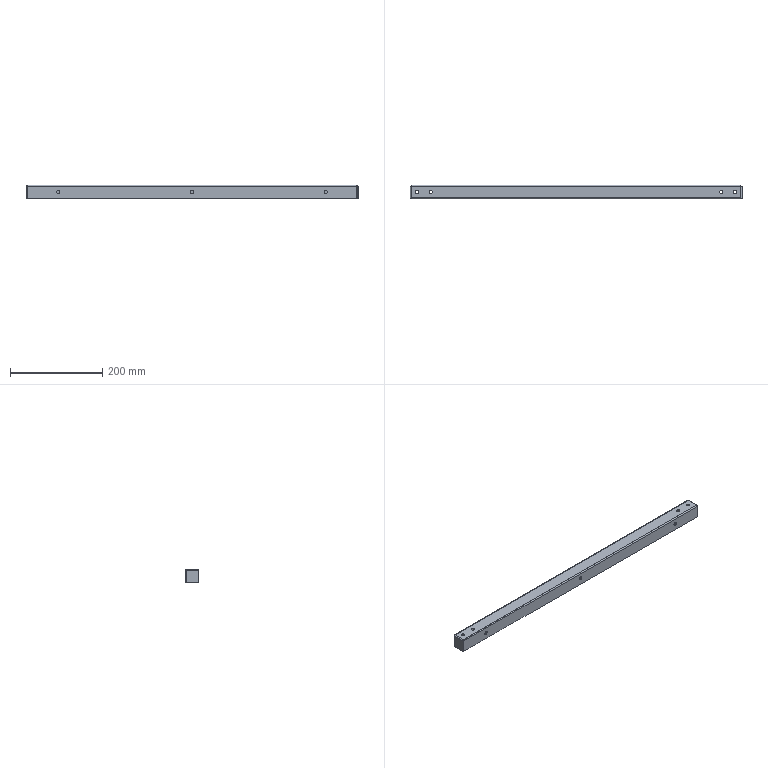Part | STEP file | Front lower sheet metal baffle | 1 solid | 54 faces | box 720 x 30 x 30 mm | volume 93839 mm3 | plane 28 | cylinder 22 | spline 4 | commonest cylinder face diameters 7 x14 2 x4 5 x4